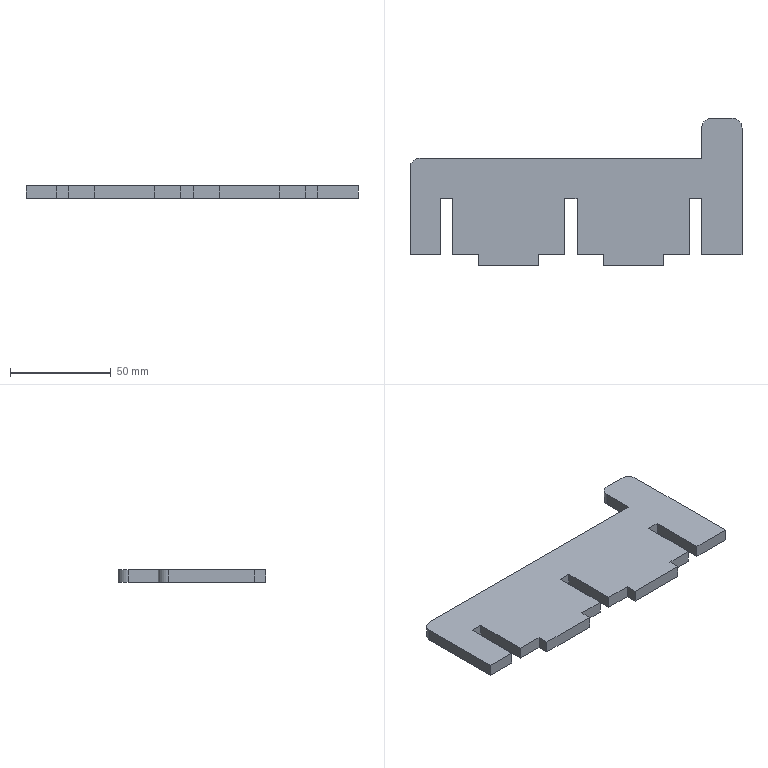Part | SolidWorks | features Fillet 1, FlatPattern 1, SMBaseFlange 1, SheetMetal 1 | 1 solid | 31 faces | box 165 x 73.5 x 6 mm | volume 48779 mm3 | plane 28 | cylinder 3 | commonest cylinder face diameters 10 x3
STEP:
#1=CARTESIAN_POINT('',(-103.903,-259.,0.));
#2=VERTEX_POINT('',#1);
#3=CARTESIAN_POINT('',(-88.903,-259.,0.));
#4=VERTEX_POINT('',#3);
#5=CARTESIAN_POINT('',(-88.903,-259.,0.));
#6=DIRECTION('',(1.,0.,0.));
#7=VECTOR('',#6,1000.);
#8=LINE('',#5,#7);
#9=EDGE_CURVE('',#2,#4,#8,.T.);
#10=ORIENTED_EDGE('',*,*,#9,.F.);
#11=CARTESIAN_POINT('',(-103.903,-259.,-6.));
#12=VERTEX_POINT('',#11);
#13=CARTESIAN_POINT('',(-103.903,-259.,-6.));
#14=DIRECTION('',(0.,0.,1.));
#15=VECTOR('',#14,1000.);
#16=LINE('',#13,#15);
#17=EDGE_CURVE('',#12,#2,#16,.T.);
#18=ORIENTED_EDGE('',*,*,#17,.F.);
#19=CARTESIAN_POINT('',(-88.903,-259.,-6.));
#20=VERTEX_POINT('',#19);
#21=CARTESIAN_POINT('',(-88.903,-259.,-6.));
#22=DIRECTION('',(1.,0.,0.));
#23=VECTOR('',#22,1000.);
#24=LINE('',#21,#23);
#25=EDGE_CURVE('',#12,#20,#24,.T.);
#26=ORIENTED_EDGE('',*,*,#25,.T.);
#27=CARTESIAN_POINT('',(-88.903,-259.,-6.));
#28=DIRECTION('',(0.,0.,1.));
#29=VECTOR('',#28,1000.);
#30=LINE('',#27,#29);
#31=EDGE_CURVE('',#20,#4,#30,.T.);
#32=ORIENTED_EDGE('',*,*,#31,.T.);
#33=EDGE_LOOP('',(#10,#18,#26,#32));
#34=FACE_OUTER_BOUND('',#33,.T.);
#35=CARTESIAN_POINT('',(-88.903,-259.,-6.));
#36=DIRECTION('',(0.,-1.,0.));
#37=DIRECTION('',(1.,0.,0.));
#38=AXIS2_PLACEMENT_3D('',#35,#36,#37);
#39=PLANE('',#38);
#40=ADVANCED_FACE('',(#34),#39,.T.);
#41=CARTESIAN_POINT('',(-103.903,-216.,0.));
#42=VERTEX_POINT('',#41);
#43=CARTESIAN_POINT('',(-103.903,-259.,0.));
#44=DIRECTION('',(0.,-1.,0.));
#45=VECTOR('',#44,1000.);
#46=LINE('',#43,#45);
#47=EDGE_CURVE('',#42,#2,#46,.T.);
#48=ORIENTED_EDGE('',*,*,#47,.F.);
#49=CARTESIAN_POINT('',(-103.903,-216.,-6.));
#50=VERTEX_POINT('',#49);
#51=CARTESIAN_POINT('',(-103.903,-216.,-6.));
#52=DIRECTION('',(0.,0.,-1.));
#53=VECTOR('',#52,1000.);
#54=LINE('',#51,#53);
#55=EDGE_CURVE('',#42,#50,#54,.T.);
#56=ORIENTED_EDGE('',*,*,#55,.T.);
#57=CARTESIAN_POINT('',(-103.903,-259.,-6.));
#58=DIRECTION('',(0.,-1.,0.));
#59=VECTOR('',#58,1000.);
#60=LINE('',#57,#59);
#61=EDGE_CURVE('',#50,#12,#60,.T.);
#62=ORIENTED_EDGE('',*,*,#61,.T.);
#63=ORIENTED_EDGE('',*,*,#17,.T.);
#64=EDGE_LOOP('',(#48,#56,#62,#63));
#65=FACE_OUTER_BOUND('',#64,.T.);
#66=CARTESIAN_POINT('',(-103.903,-259.,-6.));
#67=DIRECTION('',(-1.,0.,0.));
#68=DIRECTION('',(0.,0.,1.));
#69=AXIS2_PLACEMENT_3D('',#66,#67,#68);
#70=PLANE('',#69);
#71=ADVANCED_FACE('',(#65),#70,.T.);
#72=CARTESIAN_POINT('',(41.097,-211.,-6.));
#73=VERTEX_POINT('',#72);
#74=CARTESIAN_POINT('',(-98.903,-211.,-6.));
#75=VERTEX_POINT('',#74);
#76=CARTESIAN_POINT('',(-103.903,-211.,-6.));
#77=DIRECTION('',(-1.,0.,0.));
#78=VECTOR('',#77,1000.);
#79=LINE('',#76,#78);
#80=EDGE_CURVE('',#73,#75,#79,.T.);
#81=ORIENTED_EDGE('',*,*,#80,.T.);
#82=CARTESIAN_POINT('',(-98.903,-211.,0.));
#83=VERTEX_POINT('',#82);
#84=CARTESIAN_POINT('',(-98.903,-211.,-6.));
#85=DIRECTION('',(0.,0.,1.));
#86=VECTOR('',#85,1000.);
#87=LINE('',#84,#86);
#88=EDGE_CURVE('',#75,#83,#87,.T.);
#89=ORIENTED_EDGE('',*,*,#88,.T.);
#90=CARTESIAN_POINT('',(41.097,-211.,0.));
#91=VERTEX_POINT('',#90);
#92=CARTESIAN_POINT('',(-103.903,-211.,0.));
#93=DIRECTION('',(-1.,0.,0.));
#94=VECTOR('',#93,1000.);
#95=LINE('',#92,#94);
#96=EDGE_CURVE('',#91,#83,#95,.T.);
#97=ORIENTED_EDGE('',*,*,#96,.F.);
#98=CARTESIAN_POINT('',(41.097,-211.,-6.));
#99=DIRECTION('',(0.,0.,1.));
#100=VECTOR('',#99,1000.);
#101=LINE('',#98,#100);
#102=EDGE_CURVE('',#73,#91,#101,.T.);
#103=ORIENTED_EDGE('',*,*,#102,.F.);
#104=EDGE_LOOP('',(#81,#89,#97,#103));
#105=FACE_OUTER_BOUND('',#104,.T.);
#106=CARTESIAN_POINT('',(-103.903,-211.,-6.));
#107=DIRECTION('',(0.,1.,0.));
#108=DIRECTION('',(0.,0.,1.));
#109=AXIS2_PLACEMENT_3D('',#106,#107,#108);
#110=PLANE('',#109);
#111=ADVANCED_FACE('',(#105),#110,.T.);
#112=CARTESIAN_POINT('',(41.097,-196.,0.));
#113=VERTEX_POINT('',#112);
#114=CARTESIAN_POINT('',(41.097,-211.,0.));
#115=DIRECTION('',(0.,-1.,0.));
#116=VECTOR('',#115,1000.);
#117=LINE('',#114,#116);
#118=EDGE_CURVE('',#113,#91,#117,.T.);
#119=ORIENTED_EDGE('',*,*,#118,.F.);
#120=CARTESIAN_POINT('',(41.097,-196.,-6.));
#121=VERTEX_POINT('',#120);
#122=CARTESIAN_POINT('',(41.097,-196.,-6.));
#123=DIRECTION('',(0.,0.,-1.));
#124=VECTOR('',#123,1000.);
#125=LINE('',#122,#124);
#126=EDGE_CURVE('',#113,#121,#125,.T.);
#127=ORIENTED_EDGE('',*,*,#126,.T.);
#128=CARTESIAN_POINT('',(41.097,-211.,-6.));
#129=DIRECTION('',(0.,-1.,0.));
#130=VECTOR('',#129,1000.);
#131=LINE('',#128,#130);
#132=EDGE_CURVE('',#121,#73,#131,.T.);
#133=ORIENTED_EDGE('',*,*,#132,.T.);
#134=ORIENTED_EDGE('',*,*,#102,.T.);
#135=EDGE_LOOP('',(#119,#127,#133,#134));
#136=FACE_OUTER_BOUND('',#135,.T.);
#137=CARTESIAN_POINT('',(41.097,-211.,-6.));
#138=DIRECTION('',(-1.,0.,0.));
#139=DIRECTION('',(0.,-1.,0.));
#140=AXIS2_PLACEMENT_3D('',#137,#138,#139);
#141=PLANE('',#140);
#142=ADVANCED_FACE('',(#136),#141,.T.);
#143=CARTESIAN_POINT('',(56.097,-191.,0.));
#144=VERTEX_POINT('',#143);
#145=CARTESIAN_POINT('',(46.097,-191.,0.));
#146=VERTEX_POINT('',#145);
#147=CARTESIAN_POINT('',(41.097,-191.,0.));
#148=DIRECTION('',(-1.,0.,0.));
#149=VECTOR('',#148,1000.);
#150=LINE('',#147,#149);
#151=EDGE_CURVE('',#144,#146,#150,.T.);
#152=ORIENTED_EDGE('',*,*,#151,.F.);
#153=CARTESIAN_POINT('',(56.097,-191.,-6.));
#154=VERTEX_POINT('',#153);
#155=CARTESIAN_POINT('',(56.097,-191.,-6.));
#156=DIRECTION('',(0.,0.,-1.));
#157=VECTOR('',#156,1000.);
#158=LINE('',#155,#157);
#159=EDGE_CURVE('',#144,#154,#158,.T.);
#160=ORIENTED_EDGE('',*,*,#159,.T.);
#161=CARTESIAN_POINT('',(46.097,-191.,-6.));
#162=VERTEX_POINT('',#161);
#163=CARTESIAN_POINT('',(41.097,-191.,-6.));
#164=DIRECTION('',(-1.,0.,0.));
#165=VECTOR('',#164,1000.);
#166=LINE('',#163,#165);
#167=EDGE_CURVE('',#154,#162,#166,.T.);
#168=ORIENTED_EDGE('',*,*,#167,.T.);
#169=CARTESIAN_POINT('',(46.097,-191.,-6.));
#170=DIRECTION('',(0.,0.,1.));
#171=VECTOR('',#170,1000.);
#172=LINE('',#169,#171);
#173=EDGE_CURVE('',#162,#146,#172,.T.);
#174=ORIENTED_EDGE('',*,*,#173,.T.);
#175=EDGE_LOOP('',(#152,#160,#168,#174));
#176=FACE_OUTER_BOUND('',#175,.T.);
#177=CARTESIAN_POINT('',(41.097,-191.,-6.));
#178=DIRECTION('',(0.,1.,0.));
#179=DIRECTION('',(0.,0.,1.));
#180=AXIS2_PLACEMENT_3D('',#177,#178,#179);
#181=PLANE('',#180);
#182=ADVANCED_FACE('',(#176),#181,.T.);
#183=CARTESIAN_POINT('',(61.097,-259.,-6.));
#184=VERTEX_POINT('',#183);
#185=CARTESIAN_POINT('',(61.097,-196.,-6.));
#186=VERTEX_POINT('',#185);
#187=CARTESIAN_POINT('',(61.097,-191.,-6.));
#188=DIRECTION('',(0.,1.,0.));
#189=VECTOR('',#188,1000.);
#190=LINE('',#187,#189);
#191=EDGE_CURVE('',#184,#186,#190,.T.);
#192=ORIENTED_EDGE('',*,*,#191,.T.);
#193=CARTESIAN_POINT('',(61.097,-196.,0.));
#194=VERTEX_POINT('',#193);
#195=CARTESIAN_POINT('',(61.097,-196.,-6.));
#196=DIRECTION('',(0.,0.,1.));
#197=VECTOR('',#196,1000.);
#198=LINE('',#195,#197);
#199=EDGE_CURVE('',#186,#194,#198,.T.);
#200=ORIENTED_EDGE('',*,*,#199,.T.);
#201=CARTESIAN_POINT('',(61.097,-259.,0.));
#202=VERTEX_POINT('',#201);
#203=CARTESIAN_POINT('',(61.097,-191.,0.));
#204=DIRECTION('',(0.,1.,0.));
#205=VECTOR('',#204,1000.);
#206=LINE('',#203,#205);
#207=EDGE_CURVE('',#202,#194,#206,.T.);
#208=ORIENTED_EDGE('',*,*,#207,.F.);
#209=CARTESIAN_POINT('',(61.097,-259.,-6.));
#210=DIRECTION('',(0.,0.,1.));
#211=VECTOR('',#210,1000.);
#212=LINE('',#209,#211);
#213=EDGE_CURVE('',#184,#202,#212,.T.);
#214=ORIENTED_EDGE('',*,*,#213,.F.);
#215=EDGE_LOOP('',(#192,#200,#208,#214));
#216=FACE_OUTER_BOUND('',#215,.T.);
#217=CARTESIAN_POINT('',(61.097,-191.,-6.));
#218=DIRECTION('',(1.,0.,0.));
#219=DIRECTION('',(0.,1.,0.));
#220=AXIS2_PLACEMENT_3D('',#217,#218,#219);
#221=PLANE('',#220);
#222=ADVANCED_FACE('',(#216),#221,.T.);
#223=CARTESIAN_POINT('',(41.097,-259.,0.));
#224=VERTEX_POINT('',#223);
#225=CARTESIAN_POINT('',(61.097,-259.,0.));
#226=DIRECTION('',(1.,0.,0.));
#227=VECTOR('',#226,1000.);
#228=LINE('',#225,#227);
#229=EDGE_CURVE('',#224,#202,#228,.T.);
#230=ORIENTED_EDGE('',*,*,#229,.F.);
#231=CARTESIAN_POINT('',(41.097,-259.,-6.));
#232=VERTEX_POINT('',#231);
#233=CARTESIAN_POINT('',(41.097,-259.,-6.));
#234=DIRECTION('',(0.,0.,1.));
#235=VECTOR('',#234,1000.);
#236=LINE('',#233,#235);
#237=EDGE_CURVE('',#232,#224,#236,.T.);
#238=ORIENTED_EDGE('',*,*,#237,.F.);
#239=CARTESIAN_POINT('',(61.097,-259.,-6.));
#240=DIRECTION('',(1.,0.,0.));
#241=VECTOR('',#240,1000.);
#242=LINE('',#239,#241);
#243=EDGE_CURVE('',#232,#184,#242,.T.);
#244=ORIENTED_EDGE('',*,*,#243,.T.);
#245=ORIENTED_EDGE('',*,*,#213,.T.);
#246=EDGE_LOOP('',(#230,#238,#244,#245));
#247=FACE_OUTER_BOUND('',#246,.T.);
#248=CARTESIAN_POINT('',(61.097,-259.,-6.));
#249=DIRECTION('',(0.,-1.,0.));
#250=DIRECTION('',(1.,0.,0.));
#251=AXIS2_PLACEMENT_3D('',#248,#249,#250);
#252=PLANE('',#251);
#253=ADVANCED_FACE('',(#247),#252,.T.);
#254=CARTESIAN_POINT('',(41.097,-231.,0.));
#255=VERTEX_POINT('',#254);
#256=CARTESIAN_POINT('',(41.097,-231.,0.));
#257=DIRECTION('',(0.,-1.,0.));
#258=VECTOR('',#257,1000.);
#259=LINE('',#256,#258);
#260=EDGE_CURVE('',#255,#224,#259,.T.);
#261=ORIENTED_EDGE('',*,*,#260,.F.);
#262=CARTESIAN_POINT('',(41.097,-231.,-6.));
#263=VERTEX_POINT('',#262);
#264=CARTESIAN_POINT('',(41.097,-231.,-6.));
#265=DIRECTION('',(0.,0.,1.));
#266=VECTOR('',#265,1000.);
#267=LINE('',#264,#266);
#268=EDGE_CURVE('',#263,#255,#267,.T.);
#269=ORIENTED_EDGE('',*,*,#268,.F.);
#270=CARTESIAN_POINT('',(41.097,-231.,-6.));
#271=DIRECTION('',(0.,-1.,0.));
#272=VECTOR('',#271,1000.);
#273=LINE('',#270,#272);
#274=EDGE_CURVE('',#263,#232,#273,.T.);
#275=ORIENTED_EDGE('',*,*,#274,.T.);
#276=ORIENTED_EDGE('',*,*,#237,.T.);
#277=EDGE_LOOP('',(#261,#269,#275,#276));
#278=FACE_OUTER_BOUND('',#277,.T.);
#279=CARTESIAN_POINT('',(41.097,-231.,-6.));
#280=DIRECTION('',(-1.,0.,0.));
#281=DIRECTION('',(0.,-1.,0.));
#282=AXIS2_PLACEMENT_3D('',#279,#280,#281);
#283=PLANE('',#282);
#284=ADVANCED_FACE('',(#278),#283,.T.);
#285=CARTESIAN_POINT('',(35.097,-231.,0.));
#286=VERTEX_POINT('',#285);
#287=CARTESIAN_POINT('',(35.097,-231.,0.));
#288=DIRECTION('',(1.,0.,0.));
#289=VECTOR('',#288,1000.);
#290=LINE('',#287,#289);
#291=EDGE_CURVE('',#286,#255,#290,.T.);
#292=ORIENTED_EDGE('',*,*,#291,.F.);
#293=CARTESIAN_POINT('',(35.097,-231.,-6.));
#294=VERTEX_POINT('',#293);
#295=CARTESIAN_POINT('',(35.097,-231.,-6.));
#296=DIRECTION('',(0.,0.,1.));
#297=VECTOR('',#296,1000.);
#298=LINE('',#295,#297);
#299=EDGE_CURVE('',#294,#286,#298,.T.);
#300=ORIENTED_EDGE('',*,*,#299,.F.);
#301=CARTESIAN_POINT('',(35.097,-231.,-6.));
#302=DIRECTION('',(1.,0.,0.));
#303=VECTOR('',#302,1000.);
#304=LINE('',#301,#303);
#305=EDGE_CURVE('',#294,#263,#304,.T.);
#306=ORIENTED_EDGE('',*,*,#305,.T.);
#307=ORIENTED_EDGE('',*,*,#268,.T.);
#308=EDGE_LOOP('',(#292,#300,#306,#307));
#309=FACE_OUTER_BOUND('',#308,.T.);
#310=CARTESIAN_POINT('',(35.097,-231.,-6.));
#311=DIRECTION('',(0.,-1.,0.));
#312=DIRECTION('',(1.,0.,0.));
#313=AXIS2_PLACEMENT_3D('',#310,#311,#312);
#314=PLANE('',#313);
#315=ADVANCED_FACE('',(#309),#314,.T.);
#316=CARTESIAN_POINT('',(35.097,-259.,0.));
#317=VERTEX_POINT('',#316);
#318=CARTESIAN_POINT('',(35.097,-259.,0.));
#319=DIRECTION('',(0.,1.,0.));
#320=VECTOR('',#319,1000.);
#321=LINE('',#318,#320);
#322=EDGE_CURVE('',#317,#286,#321,.T.);
#323=ORIENTED_EDGE('',*,*,#322,.F.);
#324=CARTESIAN_POINT('',(35.097,-259.,-6.));
#325=VERTEX_POINT('',#324);
#326=CARTESIAN_POINT('',(35.097,-259.,-6.));
#327=DIRECTION('',(0.,0.,1.));
#328=VECTOR('',#327,1000.);
#329=LINE('',#326,#328);
#330=EDGE_CURVE('',#325,#317,#329,.T.);
#331=ORIENTED_EDGE('',*,*,#330,.F.);
#332=CARTESIAN_POINT('',(35.097,-259.,-6.));
#333=DIRECTION('',(0.,1.,0.));
#334=VECTOR('',#333,1000.);
#335=LINE('',#332,#334);
#336=EDGE_CURVE('',#325,#294,#335,.T.);
#337=ORIENTED_EDGE('',*,*,#336,.T.);
#338=ORIENTED_EDGE('',*,*,#299,.T.);
#339=EDGE_LOOP('',(#323,#331,#337,#338));
#340=FACE_OUTER_BOUND('',#339,.T.);
#341=CARTESIAN_POINT('',(35.097,-259.,-6.));
#342=DIRECTION('',(1.,0.,0.));
#343=DIRECTION('',(0.,1.,0.));
#344=AXIS2_PLACEMENT_3D('',#341,#342,#343);
#345=PLANE('',#344);
#346=ADVANCED_FACE('',(#340),#345,.T.);
#347=CARTESIAN_POINT('',(22.097,-259.,0.));
#348=VERTEX_POINT('',#347);
#349=CARTESIAN_POINT('',(35.097,-259.,0.));
#350=DIRECTION('',(1.,0.,0.));
#351=VECTOR('',#350,1000.);
#352=LINE('',#349,#351);
#353=EDGE_CURVE('',#348,#317,#352,.T.);
#354=ORIENTED_EDGE('',*,*,#353,.F.);
#355=CARTESIAN_POINT('',(22.097,-259.,-6.));
#356=VERTEX_POINT('',#355);
#357=CARTESIAN_POINT('',(22.097,-259.,-6.));
#358=DIRECTION('',(0.,0.,1.));
#359=VECTOR('',#358,1000.);
#360=LINE('',#357,#359);
#361=EDGE_CURVE('',#356,#348,#360,.T.);
#362=ORIENTED_EDGE('',*,*,#361,.F.);
#363=CARTESIAN_POINT('',(35.097,-259.,-6.));
#364=DIRECTION('',(1.,0.,0.));
#365=VECTOR('',#364,1000.);
#366=LINE('',#363,#365);
#367=EDGE_CURVE('',#356,#325,#366,.T.);
#368=ORIENTED_EDGE('',*,*,#367,.T.);
#369=ORIENTED_EDGE('',*,*,#330,.T.);
#370=EDGE_LOOP('',(#354,#362,#368,#369));
#371=FACE_OUTER_BOUND('',#370,.T.);
#372=CARTESIAN_POINT('',(35.097,-259.,-6.));
#373=DIRECTION('',(0.,-1.,0.));
#374=DIRECTION('',(0.,0.,-1.));
#375=AXIS2_PLACEMENT_3D('',#372,#373,#374);
#376=PLANE('',#375);
#377=ADVANCED_FACE('',(#371),#376,.T.);
#378=CARTESIAN_POINT('',(22.097,-264.5,0.));
#379=VERTEX_POINT('',#378);
#380=CARTESIAN_POINT('',(22.097,-264.5,0.));
#381=DIRECTION('',(0.,1.,0.));
#382=VECTOR('',#381,1000.);
#383=LINE('',#380,#382);
#384=EDGE_CURVE('',#379,#348,#383,.T.);
#385=ORIENTED_EDGE('',*,*,#384,.F.);
#386=CARTESIAN_POINT('',(22.097,-264.5,-6.));
#387=VERTEX_POINT('',#386);
#388=CARTESIAN_POINT('',(22.097,-264.5,-6.));
#389=DIRECTION('',(0.,0.,1.));
#390=VECTOR('',#389,1000.);
#391=LINE('',#388,#390);
#392=EDGE_CURVE('',#387,#379,#391,.T.);
#393=ORIENTED_EDGE('',*,*,#392,.F.);
#394=CARTESIAN_POINT('',(22.097,-264.5,-6.));
#395=DIRECTION('',(0.,1.,0.));
#396=VECTOR('',#395,1000.);
#397=LINE('',#394,#396);
#398=EDGE_CURVE('',#387,#356,#397,.T.);
#399=ORIENTED_EDGE('',*,*,#398,.T.);
#400=ORIENTED_EDGE('',*,*,#361,.T.);
#401=EDGE_LOOP('',(#385,#393,#399,#400));
#402=FACE_OUTER_BOUND('',#401,.T.);
#403=CARTESIAN_POINT('',(22.097,-264.5,-6.));
#404=DIRECTION('',(1.,0.,0.));
#405=DIRECTION('',(0.,0.,-1.));
#406=AXIS2_PLACEMENT_3D('',#403,#404,#405);
#407=PLANE('',#406);
#408=ADVANCED_FACE('',(#402),#407,.T.);
#409=CARTESIAN_POINT('',(-7.903,-264.5,0.));
#410=VERTEX_POINT('',#409);
#411=CARTESIAN_POINT('',(-7.903,-264.5,0.));
#412=DIRECTION('',(1.,0.,0.));
#413=VECTOR('',#412,1000.);
#414=LINE('',#411,#413);
#415=EDGE_CURVE('',#410,#379,#414,.T.);
#416=ORIENTED_EDGE('',*,*,#415,.F.);
#417=CARTESIAN_POINT('',(-7.903,-264.5,-6.));
#418=VERTEX_POINT('',#417);
#419=CARTESIAN_POINT('',(-7.903,-264.5,-6.));
#420=DIRECTION('',(0.,0.,1.));
#421=VECTOR('',#420,1000.);
#422=LINE('',#419,#421);
#423=EDGE_CURVE('',#418,#410,#422,.T.);
#424=ORIENTED_EDGE('',*,*,#423,.F.);
#425=CARTESIAN_POINT('',(-7.903,-264.5,-6.));
#426=DIRECTION('',(1.,0.,0.));
#427=VECTOR('',#426,1000.);
#428=LINE('',#425,#427);
#429=EDGE_CURVE('',#418,#387,#428,.T.);
#430=ORIENTED_EDGE('',*,*,#429,.T.);
#431=ORIENTED_EDGE('',*,*,#392,.T.);
#432=EDGE_LOOP('',(#416,#424,#430,#431));
#433=FACE_OUTER_BOUND('',#432,.T.);
#434=CARTESIAN_POINT('',(-7.903,-264.5,-6.));
#435=DIRECTION('',(0.,-1.,0.));
#436=DIRECTION('',(0.,0.,-1.));
#437=AXIS2_PLACEMENT_3D('',#434,#435,#436);
#438=PLANE('',#437);
#439=ADVANCED_FACE('',(#433),#438,.T.);
#440=CARTESIAN_POINT('',(-7.903,-259.,0.));
#441=VERTEX_POINT('',#440);
#442=CARTESIAN_POINT('',(-7.903,-259.,0.));
#443=DIRECTION('',(0.,-1.,0.));
#444=VECTOR('',#443,1000.);
#445=LINE('',#442,#444);
#446=EDGE_CURVE('',#441,#410,#445,.T.);
#447=ORIENTED_EDGE('',*,*,#446,.F.);
#448=CARTESIAN_POINT('',(-7.903,-259.,-6.));
#449=VERTEX_POINT('',#448);
#450=CARTESIAN_POINT('',(-7.903,-259.,-6.));
#451=DIRECTION('',(0.,0.,1.));
#452=VECTOR('',#451,1000.);
#453=LINE('',#450,#452);
#454=EDGE_CURVE('',#449,#441,#453,.T.);
#455=ORIENTED_EDGE('',*,*,#454,.F.);
#456=CARTESIAN_POINT('',(-7.903,-259.,-6.));
#457=DIRECTION('',(0.,-1.,0.));
#458=VECTOR('',#457,1000.);
#459=LINE('',#456,#458);
#460=EDGE_CURVE('',#449,#418,#459,.T.);
#461=ORIENTED_EDGE('',*,*,#460,.T.);
#462=ORIENTED_EDGE('',*,*,#423,.T.);
#463=EDGE_LOOP('',(#447,#455,#461,#462));
#464=FACE_OUTER_BOUND('',#463,.T.);
#465=CARTESIAN_POINT('',(-7.903,-259.,-6.));
#466=DIRECTION('',(-1.,0.,0.));
#467=DIRECTION('',(0.,0.,1.));
#468=AXIS2_PLACEMENT_3D('',#465,#466,#467);
#469=PLANE('',#468);
#470=ADVANCED_FACE('',(#464),#469,.T.);
#471=CARTESIAN_POINT('',(-20.903,-259.,0.));
#472=VERTEX_POINT('',#471);
#473=CARTESIAN_POINT('',(-7.903,-259.,0.));
#474=DIRECTION('',(1.,0.,0.));
#475=VECTOR('',#474,1000.);
#476=LINE('',#473,#475);
#477=EDGE_CURVE('',#472,#441,#476,.T.);
#478=ORIENTED_EDGE('',*,*,#477,.F.);
#479=CARTESIAN_POINT('',(-20.903,-259.,-6.));
#480=VERTEX_POINT('',#479);
#481=CARTESIAN_POINT('',(-20.903,-259.,-6.));
#482=DIRECTION('',(0.,0.,1.));
#483=VECTOR('',#482,1000.);
#484=LINE('',#481,#483);
#485=EDGE_CURVE('',#480,#472,#484,.T.);
#486=ORIENTED_EDGE('',*,*,#485,.F.);
#487=CARTESIAN_POINT('',(-7.903,-259.,-6.));
#488=DIRECTION('',(1.,0.,0.));
#489=VECTOR('',#488,1000.);
#490=LINE('',#487,#489);
#491=EDGE_CURVE('',#480,#449,#490,.T.);
#492=ORIENTED_EDGE('',*,*,#491,.T.);
#493=ORIENTED_EDGE('',*,*,#454,.T.);
#494=EDGE_LOOP('',(#478,#486,#492,#493));
#495=FACE_OUTER_BOUND('',#494,.T.);
#496=CARTESIAN_POINT('',(-7.903,-259.,-6.));
#497=DIRECTION('',(0.,-1.,0.));
#498=DIRECTION('',(1.,0.,0.));
#499=AXIS2_PLACEMENT_3D('',#496,#497,#498);
#500=PLANE('',#499);
#501=ADVANCED_FACE('',(#495),#500,.T.);
#502=CARTESIAN_POINT('',(-20.903,-231.,0.));
#503=VERTEX_POINT('',#502);
#504=CARTESIAN_POINT('',(-20.903,-231.,0.));
#505=DIRECTION('',(0.,-1.,0.));
#506=VECTOR('',#505,1000.);
#507=LINE('',#504,#506);
#508=EDGE_CURVE('',#503,#472,#507,.T.);
#509=ORIENTED_EDGE('',*,*,#508,.F.);
#510=CARTESIAN_POINT('',(-20.903,-231.,-6.));
#511=VERTEX_POINT('',#510);
#512=CARTESIAN_POINT('',(-20.903,-231.,-6.));
#513=DIRECTION('',(0.,0.,1.));
#514=VECTOR('',#513,1000.);
#515=LINE('',#512,#514);
#516=EDGE_CURVE('',#511,#503,#515,.T.);
#517=ORIENTED_EDGE('',*,*,#516,.F.);
#518=CARTESIAN_POINT('',(-20.903,-231.,-6.));
#519=DIRECTION('',(0.,-1.,0.));
#520=VECTOR('',#519,1000.);
#521=LINE('',#518,#520);
#522=EDGE_CURVE('',#511,#480,#521,.T.);
#523=ORIENTED_EDGE('',*,*,#522,.T.);
#524=ORIENTED_EDGE('',*,*,#485,.T.);
#525=EDGE_LOOP('',(#509,#517,#523,#524));
#526=FACE_OUTER_BOUND('',#525,.T.);
#527=CARTESIAN_POINT('',(-20.903,-231.,-6.));
#528=DIRECTION('',(-1.,0.,0.));
#529=DIRECTION('',(0.,-1.,0.));
#530=AXIS2_PLACEMENT_3D('',#527,#528,#529);
#531=PLANE('',#530);
#532=ADVANCED_FACE('',(#526),#531,.T.);
#533=CARTESIAN_POINT('',(-26.903,-231.,0.));
#534=VERTEX_POINT('',#533);
#535=CARTESIAN_POINT('',(-26.903,-231.,0.));
#536=DIRECTION('',(1.,0.,0.));
#537=VECTOR('',#536,1000.);
#538=LINE('',#535,#537);
#539=EDGE_CURVE('',#534,#503,#538,.T.);
#540=ORIENTED_EDGE('',*,*,#539,.F.);
#541=CARTESIAN_POINT('',(-26.903,-231.,-6.));
#542=VERTEX_POINT('',#541);
#543=CARTESIAN_POINT('',(-26.903,-231.,-6.));
#544=DIRECTION('',(0.,0.,1.));
#545=VECTOR('',#544,1000.);
#546=LINE('',#543,#545);
#547=EDGE_CURVE('',#542,#534,#546,.T.);
#548=ORIENTED_EDGE('',*,*,#547,.F.);
#549=CARTESIAN_POINT('',(-26.903,-231.,-6.));
#550=DIRECTION('',(1.,0.,0.));
#551=VECTOR('',#550,1000.);
#552=LINE('',#549,#551);
#553=EDGE_CURVE('',#542,#511,#552,.T.);
#554=ORIENTED_EDGE('',*,*,#553,.T.);
#555=ORIENTED_EDGE('',*,*,#516,.T.);
#556=EDGE_LOOP('',(#540,#548,#554,#555));
#557=FACE_OUTER_BOUND('',#556,.T.);
#558=CARTESIAN_POINT('',(-26.903,-231.,-6.));
#559=DIRECTION('',(0.,-1.,0.));
#560=DIRECTION('',(0.,0.,-1.));
#561=AXIS2_PLACEMENT_3D('',#558,#559,#560);
#562=PLANE('',#561);
#563=ADVANCED_FACE('',(#557),#562,.T.);
#564=CARTESIAN_POINT('',(-26.903,-259.,0.));
#565=VERTEX_POINT('',#564);
#566=CARTESIAN_POINT('',(-26.903,-259.,0.));
#567=DIRECTION('',(0.,1.,0.));
#568=VECTOR('',#567,1000.);
#569=LINE('',#566,#568);
#570=EDGE_CURVE('',#565,#534,#569,.T.);
#571=ORIENTED_EDGE('',*,*,#570,.F.);
#572=CARTESIAN_POINT('',(-26.903,-259.,-6.));
#573=VERTEX_POINT('',#572);
#574=CARTESIAN_POINT('',(-26.903,-259.,-6.));
#575=DIRECTION('',(0.,0.,1.));
#576=VECTOR('',#575,1000.);
#577=LINE('',#574,#576);
#578=EDGE_CURVE('',#573,#565,#577,.T.);
#579=ORIENTED_EDGE('',*,*,#578,.F.);
#580=CARTESIAN_POINT('',(-26.903,-259.,-6.));
#581=DIRECTION('',(0.,1.,0.));
#582=VECTOR('',#581,1000.);
#583=LINE('',#580,#582);
#584=EDGE_CURVE('',#573,#542,#583,.T.);
#585=ORIENTED_EDGE('',*,*,#584,.T.);
#586=ORIENTED_EDGE('',*,*,#547,.T.);
#587=EDGE_LOOP('',(#571,#579,#585,#586));
#588=FACE_OUTER_BOUND('',#587,.T.);
#589=CARTESIAN_POINT('',(-26.903,-259.,-6.));
#590=DIRECTION('',(1.,0.,0.));
#591=DIRECTION('',(0.,1.,0.));
#592=AXIS2_PLACEMENT_3D('',#589,#590,#591);
#593=PLANE('',#592);
#594=ADVANCED_FACE('',(#588),#593,.T.);
#595=CARTESIAN_POINT('',(-39.903,-259.,0.));
#596=VERTEX_POINT('',#595);
#597=CARTESIAN_POINT('',(-26.903,-259.,0.));
#598=DIRECTION('',(1.,0.,0.));
#599=VECTOR('',#598,1000.);
#600=LINE('',#597,#599);
#601=EDGE_CURVE('',#596,#565,#600,.T.);
#602=ORIENTED_EDGE('',*,*,#601,.F.);
#603=CARTESIAN_POINT('',(-39.903,-259.,-6.));
#604=VERTEX_POINT('',#603);
#605=CARTESIAN_POINT('',(-39.903,-259.,-6.));
#606=DIRECTION('',(0.,0.,1.));
#607=VECTOR('',#606,1000.);
#608=LINE('',#605,#607);
#609=EDGE_CURVE('',#604,#596,#608,.T.);
#610=ORIENTED_EDGE('',*,*,#609,.F.);
#611=CARTESIAN_POINT('',(-26.903,-259.,-6.));
#612=DIRECTION('',(1.,0.,0.));
#613=VECTOR('',#612,1000.);
#614=LINE('',#611,#613);
#615=EDGE_CURVE('',#604,#573,#614,.T.);
#616=ORIENTED_EDGE('',*,*,#615,.T.);
#617=ORIENTED_EDGE('',*,*,#578,.T.);
#618=EDGE_LOOP('',(#602,#610,#616,#617));
#619=FACE_OUTER_BOUND('',#618,.T.);
#620=CARTESIAN_POINT('',(-26.903,-259.,-6.));
#621=DIRECTION('',(0.,-1.,0.));
#622=DIRECTION('',(1.,0.,0.));
#623=AXIS2_PLACEMENT_3D('',#620,#621,#622);
#624=PLANE('',#623);
#625=ADVANCED_FACE('',(#619),#624,.T.);
#626=CARTESIAN_POINT('',(-39.903,-264.5,0.));
#627=VERTEX_POINT('',#626);
#628=CARTESIAN_POINT('',(-39.903,-264.5,0.));
#629=DIRECTION('',(0.,1.,0.));
#630=VECTOR('',#629,1000.);
#631=LINE('',#628,#630);
#632=EDGE_CURVE('',#627,#596,#631,.T.);
#633=ORIENTED_EDGE('',*,*,#632,.F.);
#634=CARTESIAN_POINT('',(-39.903,-264.5,-6.));
#635=VERTEX_POINT('',#634);
#636=CARTESIAN_POINT('',(-39.903,-264.5,-6.));
#637=DIRECTION('',(0.,0.,1.));
#638=VECTOR('',#637,1000.);
#639=LINE('',#636,#638);
#640=EDGE_CURVE('',#635,#627,#639,.T.);
#641=ORIENTED_EDGE('',*,*,#640,.F.);
#642=CARTESIAN_POINT('',(-39.903,-264.5,-6.));
#643=DIRECTION('',(0.,1.,0.));
#644=VECTOR('',#643,1000.);
#645=LINE('',#642,#644);
#646=EDGE_CURVE('',#635,#604,#645,.T.);
#647=ORIENTED_EDGE('',*,*,#646,.T.);
#648=ORIENTED_EDGE('',*,*,#609,.T.);
#649=EDGE_LOOP('',(#633,#641,#647,#648));
#650=FACE_OUTER_BOUND('',#649,.T.);
#651=CARTESIAN_POINT('',(-39.903,-264.5,-6.));
#652=DIRECTION('',(1.,0.,0.));
#653=DIRECTION('',(0.,0.,-1.));
#654=AXIS2_PLACEMENT_3D('',#651,#652,#653);
#655=PLANE('',#654);
#656=ADVANCED_FACE('',(#650),#655,.T.);
#657=CARTESIAN_POINT('',(-69.903,-264.5,0.));
#658=VERTEX_POINT('',#657);
#659=CARTESIAN_POINT('',(-69.903,-264.5,0.));
#660=DIRECTION('',(1.,0.,0.));
#661=VECTOR('',#660,1000.);
#662=LINE('',#659,#661);
#663=EDGE_CURVE('',#658,#627,#662,.T.);
#664=ORIENTED_EDGE('',*,*,#663,.F.);
#665=CARTESIAN_POINT('',(-69.903,-264.5,-6.));
#666=VERTEX_POINT('',#665);
#667=CARTESIAN_POINT('',(-69.903,-264.5,-6.));
#668=DIRECTION('',(0.,0.,1.));
#669=VECTOR('',#668,1000.);
#670=LINE('',#667,#669);
#671=EDGE_CURVE('',#666,#658,#670,.T.);
#672=ORIENTED_EDGE('',*,*,#671,.F.);
#673=CARTESIAN_POINT('',(-69.903,-264.5,-6.));
#674=DIRECTION('',(1.,0.,0.));
#675=VECTOR('',#674,1000.);
#676=LINE('',#673,#675);
#677=EDGE_CURVE('',#666,#635,#676,.T.);
#678=ORIENTED_EDGE('',*,*,#677,.T.);
#679=ORIENTED_EDGE('',*,*,#640,.T.);
#680=EDGE_LOOP('',(#664,#672,#678,#679));
#681=FACE_OUTER_BOUND('',#680,.T.);
#682=CARTESIAN_POINT('',(-69.903,-264.5,-6.));
#683=DIRECTION('',(0.,-1.,0.));
#684=DIRECTION('',(0.,0.,-1.));
#685=AXIS2_PLACEMENT_3D('',#682,#683,#684);
#686=PLANE('',#685);
#687=ADVANCED_FACE('',(#681),#686,.T.);
#688=CARTESIAN_POINT('',(-69.903,-259.,0.));
#689=VERTEX_POINT('',#688);
#690=CARTESIAN_POINT('',(-69.903,-259.,0.));
#691=DIRECTION('',(0.,-1.,0.));
#692=VECTOR('',#691,1000.);
#693=LINE('',#690,#692);
#694=EDGE_CURVE('',#689,#658,#693,.T.);
#695=ORIENTED_EDGE('',*,*,#694,.F.);
#696=CARTESIAN_POINT('',(-69.903,-259.,-6.));
#697=VERTEX_POINT('',#696);
#698=CARTESIAN_POINT('',(-69.903,-259.,-6.));
#699=DIRECTION('',(0.,0.,1.));
#700=VECTOR('',#699,1000.);
#701=LINE('',#698,#700);
#702=EDGE_CURVE('',#697,#689,#701,.T.);
#703=ORIENTED_EDGE('',*,*,#702,.F.);
#704=CARTESIAN_POINT('',(-69.903,-259.,-6.));
#705=DIRECTION('',(0.,-1.,0.));
#706=VECTOR('',#705,1000.);
#707=LINE('',#704,#706);
#708=EDGE_CURVE('',#697,#666,#707,.T.);
#709=ORIENTED_EDGE('',*,*,#708,.T.);
#710=ORIENTED_EDGE('',*,*,#671,.T.);
#711=EDGE_LOOP('',(#695,#703,#709,#710));
#712=FACE_OUTER_BOUND('',#711,.T.);
#713=CARTESIAN_POINT('',(-69.903,-259.,-6.));
#714=DIRECTION('',(-1.,0.,0.));
#715=DIRECTION('',(0.,-1.,0.));
#716=AXIS2_PLACEMENT_3D('',#713,#714,#715);
#717=PLANE('',#716);
#718=ADVANCED_FACE('',(#712),#717,.T.);
#719=CARTESIAN_POINT('',(-82.903,-259.,0.));
#720=VERTEX_POINT('',#719);
#721=CARTESIAN_POINT('',(-69.903,-259.,0.));
#722=DIRECTION('',(1.,0.,0.));
#723=VECTOR('',#722,1000.);
#724=LINE('',#721,#723);
#725=EDGE_CURVE('',#720,#689,#724,.T.);
#726=ORIENTED_EDGE('',*,*,#725,.F.);
#727=CARTESIAN_POINT('',(-82.903,-259.,-6.));
#728=VERTEX_POINT('',#727);
#729=CARTESIAN_POINT('',(-82.903,-259.,-6.));
#730=DIRECTION('',(0.,0.,1.));
#731=VECTOR('',#730,1000.);
#732=LINE('',#729,#731);
#733=EDGE_CURVE('',#728,#720,#732,.T.);
#734=ORIENTED_EDGE('',*,*,#733,.F.);
#735=CARTESIAN_POINT('',(-69.903,-259.,-6.));
#736=DIRECTION('',(1.,0.,0.));
#737=VECTOR('',#736,1000.);
#738=LINE('',#735,#737);
#739=EDGE_CURVE('',#728,#697,#738,.T.);
#740=ORIENTED_EDGE('',*,*,#739,.T.);
#741=ORIENTED_EDGE('',*,*,#702,.T.);
#742=EDGE_LOOP('',(#726,#734,#740,#741));
#743=FACE_OUTER_BOUND('',#742,.T.);
#744=CARTESIAN_POINT('',(-69.903,-259.,-6.));
#745=DIRECTION('',(0.,-1.,0.));
#746=DIRECTION('',(1.,0.,0.));
#747=AXIS2_PLACEMENT_3D('',#744,#745,#746);
#748=PLANE('',#747);
#749=ADVANCED_FACE('',(#743),#748,.T.);
#750=CARTESIAN_POINT('',(-82.903,-231.,0.));
#751=VERTEX_POINT('',#750);
#752=CARTESIAN_POINT('',(-82.903,-231.,0.));
#753=DIRECTION('',(0.,-1.,0.));
#754=VECTOR('',#753,1000.);
#755=LINE('',#752,#754);
#756=EDGE_CURVE('',#751,#720,#755,.T.);
#757=ORIENTED_EDGE('',*,*,#756,.F.);
#758=CARTESIAN_POINT('',(-82.903,-231.,-6.));
#759=VERTEX_POINT('',#758);
#760=CARTESIAN_POINT('',(-82.903,-231.,-6.));
#761=DIRECTION('',(0.,0.,1.));
#762=VECTOR('',#761,1000.);
#763=LINE('',#760,#762);
#764=EDGE_CURVE('',#759,#751,#763,.T.);
#765=ORIENTED_EDGE('',*,*,#764,.F.);
#766=CARTESIAN_POINT('',(-82.903,-231.,-6.));
#767=DIRECTION('',(0.,-1.,0.));
#768=VECTOR('',#767,1000.);
#769=LINE('',#766,#768);
#770=EDGE_CURVE('',#759,#728,#769,.T.);
#771=ORIENTED_EDGE('',*,*,#770,.T.);
#772=ORIENTED_EDGE('',*,*,#733,.T.);
#773=EDGE_LOOP('',(#757,#765,#771,#772));
#774=FACE_OUTER_BOUND('',#773,.T.);
#775=CARTESIAN_POINT('',(-82.903,-231.,-6.));
#776=DIRECTION('',(-1.,0.,0.));
#777=DIRECTION('',(0.,-1.,0.));
#778=AXIS2_PLACEMENT_3D('',#775,#776,#777);
#779=PLANE('',#778);
#780=ADVANCED_FACE('',(#774),#779,.T.);
#781=CARTESIAN_POINT('',(-88.903,-231.,0.));
#782=VERTEX_POINT('',#781);
#783=CARTESIAN_POINT('',(-88.903,-231.,0.));
#784=DIRECTION('',(1.,0.,0.));
#785=VECTOR('',#784,1000.);
#786=LINE('',#783,#785);
#787=EDGE_CURVE('',#782,#751,#786,.T.);
#788=ORIENTED_EDGE('',*,*,#787,.F.);
#789=CARTESIAN_POINT('',(-88.903,-231.,-6.));
#790=VERTEX_POINT('',#789);
#791=CARTESIAN_POINT('',(-88.903,-231.,-6.));
#792=DIRECTION('',(0.,0.,1.));
#793=VECTOR('',#792,1000.);
#794=LINE('',#791,#793);
#795=EDGE_CURVE('',#790,#782,#794,.T.);
#796=ORIENTED_EDGE('',*,*,#795,.F.);
#797=CARTESIAN_POINT('',(-88.903,-231.,-6.));
#798=DIRECTION('',(1.,0.,0.));
#799=VECTOR('',#798,1000.);
#800=LINE('',#797,#799);
#801=EDGE_CURVE('',#790,#759,#800,.T.);
#802=ORIENTED_EDGE('',*,*,#801,.T.);
#803=ORIENTED_EDGE('',*,*,#764,.T.);
#804=EDGE_LOOP('',(#788,#796,#802,#803));
#805=FACE_OUTER_BOUND('',#804,.T.);
#806=CARTESIAN_POINT('',(-88.903,-231.,-6.));
#807=DIRECTION('',(0.,-1.,0.));
#808=DIRECTION('',(1.,0.,0.));
#809=AXIS2_PLACEMENT_3D('',#806,#807,#808);
#810=PLANE('',#809);
#811=ADVANCED_FACE('',(#805),#810,.T.);
#812=CARTESIAN_POINT('',(-88.903,-259.,0.));
#813=DIRECTION('',(0.,1.,0.));
#814=VECTOR('',#813,1000.);
#815=LINE('',#812,#814);
#816=EDGE_CURVE('',#4,#782,#815,.T.);
#817=ORIENTED_EDGE('',*,*,#816,.F.);
#818=ORIENTED_EDGE('',*,*,#31,.F.);
#819=CARTESIAN_POINT('',(-88.903,-259.,-6.));
#820=DIRECTION('',(0.,1.,0.));
#821=VECTOR('',#820,1000.);
#822=LINE('',#819,#821);
#823=EDGE_CURVE('',#20,#790,#822,.T.);
#824=ORIENTED_EDGE('',*,*,#823,.T.);
#825=ORIENTED_EDGE('',*,*,#795,.T.);
#826=EDGE_LOOP('',(#817,#818,#824,#825));
#827=FACE_OUTER_BOUND('',#826,.T.);
#828=CARTESIAN_POINT('',(-88.903,-259.,-6.));
#829=DIRECTION('',(1.,0.,0.));
#830=DIRECTION('',(0.,1.,0.));
#831=AXIS2_PLACEMENT_3D('',#828,#829,#830);
#832=PLANE('',#831);
#833=ADVANCED_FACE('',(#827),#832,.T.);
#834=ORIENTED_EDGE('',*,*,#167,.F.);
#835=CARTESIAN_POINT('',(56.097,-196.,-6.));
#836=DIRECTION('',(0.,0.,-1.));
#837=DIRECTION('',(-1.,0.,0.));
#838=AXIS2_PLACEMENT_3D('',#835,#836,#837);
#839=CIRCLE('',#838,5.);
#840=EDGE_CURVE('',#154,#186,#839,.T.);
#841=ORIENTED_EDGE('',*,*,#840,.T.);
#842=ORIENTED_EDGE('',*,*,#191,.F.);
#843=ORIENTED_EDGE('',*,*,#243,.F.);
#844=ORIENTED_EDGE('',*,*,#274,.F.);
#845=ORIENTED_EDGE('',*,*,#305,.F.);
#846=ORIENTED_EDGE('',*,*,#336,.F.);
#847=ORIENTED_EDGE('',*,*,#367,.F.);
#848=ORIENTED_EDGE('',*,*,#398,.F.);
#849=ORIENTED_EDGE('',*,*,#429,.F.);
#850=ORIENTED_EDGE('',*,*,#460,.F.);
#851=ORIENTED_EDGE('',*,*,#491,.F.);
#852=ORIENTED_EDGE('',*,*,#522,.F.);
#853=ORIENTED_EDGE('',*,*,#553,.F.);
#854=ORIENTED_EDGE('',*,*,#584,.F.);
#855=ORIENTED_EDGE('',*,*,#615,.F.);
#856=ORIENTED_EDGE('',*,*,#646,.F.);
#857=ORIENTED_EDGE('',*,*,#677,.F.);
#858=ORIENTED_EDGE('',*,*,#708,.F.);
#859=ORIENTED_EDGE('',*,*,#739,.F.);
#860=ORIENTED_EDGE('',*,*,#770,.F.);
#861=ORIENTED_EDGE('',*,*,#801,.F.);
#862=ORIENTED_EDGE('',*,*,#823,.F.);
#863=ORIENTED_EDGE('',*,*,#25,.F.);
#864=ORIENTED_EDGE('',*,*,#61,.F.);
#865=CARTESIAN_POINT('',(-98.903,-216.,-6.));
#866=DIRECTION('',(0.,0.,-1.));
#867=DIRECTION('',(-1.,0.,0.));
#868=AXIS2_PLACEMENT_3D('',#865,#866,#867);
#869=CIRCLE('',#868,5.);
#870=EDGE_CURVE('',#50,#75,#869,.T.);
#871=ORIENTED_EDGE('',*,*,#870,.T.);
#872=ORIENTED_EDGE('',*,*,#80,.F.);
#873=ORIENTED_EDGE('',*,*,#132,.F.);
#874=CARTESIAN_POINT('',(46.097,-196.,-6.));
#875=DIRECTION('',(0.,0.,-1.));
#876=DIRECTION('',(-1.,0.,0.));
#877=AXIS2_PLACEMENT_3D('',#874,#875,#876);
#878=CIRCLE('',#877,5.);
#879=EDGE_CURVE('',#121,#162,#878,.T.);
#880=ORIENTED_EDGE('',*,*,#879,.T.);
#881=EDGE_LOOP('',(#834,#841,#842,#843,#844,#845,#846,#847,#848,#849,#850,#851,#852,#853,#854,#855,#856,#857,#858,#859,#860,#861,#862,#863,#864,#871,#872,#873,#880));
#882=FACE_OUTER_BOUND('',#881,.T.);
#883=CARTESIAN_POINT('',(0.,0.,-6.));
#884=DIRECTION('',(0.,0.,-1.));
#885=DIRECTION('',(-1.,0.,0.));
#886=AXIS2_PLACEMENT_3D('',#883,#884,#885);
#887=PLANE('',#886);
#888=ADVANCED_FACE('',(#882),#887,.T.);
#889=ORIENTED_EDGE('',*,*,#207,.T.);
#890=CARTESIAN_POINT('',(56.097,-196.,0.));
#891=DIRECTION('',(0.,0.,1.));
#892=DIRECTION('',(-1.,0.,0.));
#893=AXIS2_PLACEMENT_3D('',#890,#891,#892);
#894=CIRCLE('',#893,5.);
#895=EDGE_CURVE('',#194,#144,#894,.T.);
#896=ORIENTED_EDGE('',*,*,#895,.T.);
#897=ORIENTED_EDGE('',*,*,#151,.T.);
#898=CARTESIAN_POINT('',(46.097,-196.,0.));
#899=DIRECTION('',(0.,0.,1.));
#900=DIRECTION('',(-1.,0.,0.));
#901=AXIS2_PLACEMENT_3D('',#898,#899,#900);
#902=CIRCLE('',#901,5.);
#903=EDGE_CURVE('',#146,#113,#902,.T.);
#904=ORIENTED_EDGE('',*,*,#903,.T.);
#905=ORIENTED_EDGE('',*,*,#118,.T.);
#906=ORIENTED_EDGE('',*,*,#96,.T.);
#907=CARTESIAN_POINT('',(-98.903,-216.,0.));
#908=DIRECTION('',(0.,0.,1.));
#909=DIRECTION('',(-1.,0.,0.));
#910=AXIS2_PLACEMENT_3D('',#907,#908,#909);
#911=CIRCLE('',#910,5.);
#912=EDGE_CURVE('',#83,#42,#911,.T.);
#913=ORIENTED_EDGE('',*,*,#912,.T.);
#914=ORIENTED_EDGE('',*,*,#47,.T.);
#915=ORIENTED_EDGE('',*,*,#9,.T.);
#916=ORIENTED_EDGE('',*,*,#816,.T.);
#917=ORIENTED_EDGE('',*,*,#787,.T.);
#918=ORIENTED_EDGE('',*,*,#756,.T.);
#919=ORIENTED_EDGE('',*,*,#725,.T.);
#920=ORIENTED_EDGE('',*,*,#694,.T.);
#921=ORIENTED_EDGE('',*,*,#663,.T.);
#922=ORIENTED_EDGE('',*,*,#632,.T.);
#923=ORIENTED_EDGE('',*,*,#601,.T.);
#924=ORIENTED_EDGE('',*,*,#570,.T.);
#925=ORIENTED_EDGE('',*,*,#539,.T.);
#926=ORIENTED_EDGE('',*,*,#508,.T.);
#927=ORIENTED_EDGE('',*,*,#477,.T.);
#928=ORIENTED_EDGE('',*,*,#446,.T.);
#929=ORIENTED_EDGE('',*,*,#415,.T.);
#930=ORIENTED_EDGE('',*,*,#384,.T.);
#931=ORIENTED_EDGE('',*,*,#353,.T.);
#932=ORIENTED_EDGE('',*,*,#322,.T.);
#933=ORIENTED_EDGE('',*,*,#291,.T.);
#934=ORIENTED_EDGE('',*,*,#260,.T.);
#935=ORIENTED_EDGE('',*,*,#229,.T.);
#936=EDGE_LOOP('',(#889,#896,#897,#904,#905,#906,#913,#914,#915,#916,#917,#918,#919,#920,#921,#922,#923,#924,#925,#926,#927,#928,#929,#930,#931,#932,#933,#934,#935));
#937=FACE_OUTER_BOUND('',#936,.T.);
#938=CARTESIAN_POINT('',(0.,0.,0.));
#939=DIRECTION('',(0.,0.,-1.));
#940=DIRECTION('',(-1.,0.,0.));
#941=AXIS2_PLACEMENT_3D('',#938,#939,#940);
#942=PLANE('',#941);
#943=ADVANCED_FACE('',(#937),#942,.F.);
#944=ORIENTED_EDGE('',*,*,#840,.F.);
#945=ORIENTED_EDGE('',*,*,#159,.F.);
#946=ORIENTED_EDGE('',*,*,#895,.F.);
#947=ORIENTED_EDGE('',*,*,#199,.F.);
#948=EDGE_LOOP('',(#944,#945,#946,#947));
#949=FACE_OUTER_BOUND('',#948,.T.);
#950=CARTESIAN_POINT('',(56.097,-196.,-6.));
#951=DIRECTION('',(0.,0.,1.));
#952=DIRECTION('',(1.,0.,0.));
#953=AXIS2_PLACEMENT_3D('',#950,#951,#952);
#954=CYLINDRICAL_SURFACE('',#953,5.);
#955=ADVANCED_FACE('',(#949),#954,.T.);
#956=ORIENTED_EDGE('',*,*,#879,.F.);
#957=ORIENTED_EDGE('',*,*,#126,.F.);
#958=ORIENTED_EDGE('',*,*,#903,.F.);
#959=ORIENTED_EDGE('',*,*,#173,.F.);
#960=EDGE_LOOP('',(#956,#957,#958,#959));
#961=FACE_OUTER_BOUND('',#960,.T.);
#962=CARTESIAN_POINT('',(46.097,-196.,-6.));
#963=DIRECTION('',(0.,0.,1.));
#964=DIRECTION('',(1.,0.,0.));
#965=AXIS2_PLACEMENT_3D('',#962,#963,#964);
#966=CYLINDRICAL_SURFACE('',#965,5.);
#967=ADVANCED_FACE('',(#961),#966,.T.);
#968=ORIENTED_EDGE('',*,*,#870,.F.);
#969=ORIENTED_EDGE('',*,*,#55,.F.);
#970=ORIENTED_EDGE('',*,*,#912,.F.);
#971=ORIENTED_EDGE('',*,*,#88,.F.);
#972=EDGE_LOOP('',(#968,#969,#970,#971));
#973=FACE_OUTER_BOUND('',#972,.T.);
#974=CARTESIAN_POINT('',(-98.903,-216.,-6.));
#975=DIRECTION('',(0.,0.,1.));
#976=DIRECTION('',(1.,0.,0.));
#977=AXIS2_PLACEMENT_3D('',#974,#975,#976);
#978=CYLINDRICAL_SURFACE('',#977,5.);
#979=ADVANCED_FACE('',(#973),#978,.T.);
#980=CLOSED_SHELL('',(#40,#71,#111,#142,#182,#222,#253,#284,#315,#346,#377,#408,#439,#470,#501,#532,#563,#594,#625,#656,#687,#718,#749,#780,#811,#833,#888,#943,#955,#967,#979));
#981=MANIFOLD_SOLID_BREP('',#980);
#982=CARTESIAN_POINT('',(0.,0.,0.));
#983=DIRECTION('',(0.,0.,1.));
#984=DIRECTION('',(1.,0.,0.));
#985=AXIS2_PLACEMENT_3D('',#982,#983,#984);
#986=(LENGTH_UNIT()NAMED_UNIT(*)SI_UNIT(.MILLI.,.METRE.));
#987=UNCERTAINTY_MEASURE_WITH_UNIT(LENGTH_MEASURE(0.00001),#986,'','');
#988=(NAMED_UNIT(*)PLANE_ANGLE_UNIT()SI_UNIT($,.RADIAN.));
#989=(NAMED_UNIT(*)SI_UNIT($,.STERADIAN.)SOLID_ANGLE_UNIT());
#990=(GEOMETRIC_REPRESENTATION_CONTEXT(3)GLOBAL_UNCERTAINTY_ASSIGNED_CONTEXT((#987))GLOBAL_UNIT_ASSIGNED_CONTEXT((#986,#988,#989))REPRESENTATION_CONTEXT('',''));
#991=ADVANCED_BREP_SHAPE_REPRESENTATION('',(#981,#985),#990);